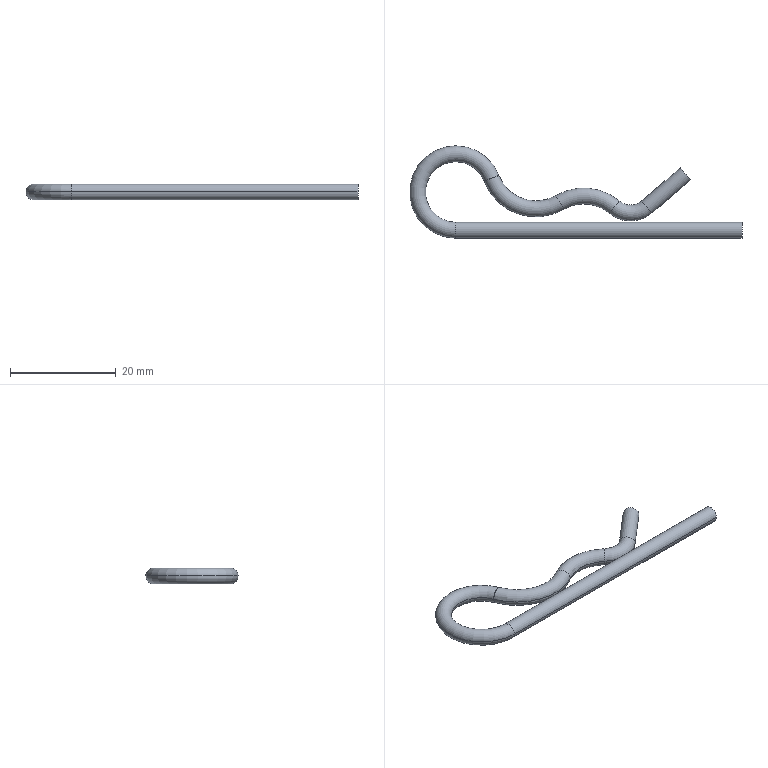Part | SolidWorks | features BaseBody 1, ICE 1, Scale 1 | 1 solid | 17 faces | box 63 x 17.5 x 3 mm | volume 910.243 mm3 | torus 8 | plane 5 | cylinder 4 | commonest cylinder face diameters 3 x4
STEP:
#1=CARTESIAN_POINT('',(9.772,3.077,0.000000307));
#2=VERTEX_POINT('',#1);
#3=CARTESIAN_POINT('',(7.84,0.7818,0.000000307));
#4=VERTEX_POINT('',#3);
#5=CARTESIAN_POINT('',(8.806,1.929,0.000000307));
#6=DIRECTION('',(0.7649,-0.6441,0.));
#7=DIRECTION('',(0.,0.,-1.));
#8=AXIS2_PLACEMENT_3D('',#5,#6,#7);
#9=CIRCLE('',#8,1.5);
#10=EDGE_CURVE('',#2,#4,#9,.T.);
#11=ORIENTED_EDGE('',*,*,#10,.T.);
#12=CARTESIAN_POINT('',(15.933,0.8171,0.000000307));
#13=VERTEX_POINT('',#12);
#14=CARTESIAN_POINT('',(11.865,5.563,0.000000307));
#15=DIRECTION('',(0.,0.,1.));
#16=DIRECTION('',(1.,0.,0.));
#17=AXIS2_PLACEMENT_3D('',#14,#15,#16);
#18=CIRCLE('',#17,6.25);
#19=EDGE_CURVE('',#4,#13,#18,.T.);
#20=ORIENTED_EDGE('',*,*,#19,.T.);
#21=CARTESIAN_POINT('',(13.98,3.095,0.000000307));
#22=VERTEX_POINT('',#21);
#23=CARTESIAN_POINT('',(14.957,1.956,0.000000307));
#24=DIRECTION('',(0.7593,0.6508,0.));
#25=DIRECTION('',(0.,0.,-1.));
#26=AXIS2_PLACEMENT_3D('',#23,#24,#25);
#27=CIRCLE('',#26,1.5);
#28=EDGE_CURVE('',#22,#13,#27,.T.);
#29=ORIENTED_EDGE('',*,*,#28,.F.);
#30=CARTESIAN_POINT('',(11.865,5.563,0.000000307));
#31=DIRECTION('',(0.,0.,1.));
#32=DIRECTION('',(1.,0.,0.));
#33=AXIS2_PLACEMENT_3D('',#30,#31,#32);
#34=CIRCLE('',#33,3.25);
#35=EDGE_CURVE('',#2,#22,#34,.T.);
#36=ORIENTED_EDGE('',*,*,#35,.F.);
#37=EDGE_LOOP('',(#11,#20,#29,#36));
#38=FACE_OUTER_BOUND('',#37,.T.);
#39=CARTESIAN_POINT('',(11.865,5.563,0.000000307));
#40=DIRECTION('',(0.,0.,1.));
#41=DIRECTION('',(-0.004363,1.,0.));
#42=AXIS2_PLACEMENT_3D('',#39,#40,#41);
#43=TOROIDAL_SURFACE('',#42,4.75,1.5);
#44=ADVANCED_FACE('',(#38),#43,.T.);
#45=CARTESIAN_POINT('',(-21.241,-0.9551,0.000000307));
#46=VERTEX_POINT('',#45);
#47=CARTESIAN_POINT('',(-21.241,-3.955,0.000000307));
#48=VERTEX_POINT('',#47);
#49=CARTESIAN_POINT('',(-21.241,-2.455,0.000000307));
#50=DIRECTION('',(-1.,0.,0.));
#51=DIRECTION('',(0.,1.,0.));
#52=AXIS2_PLACEMENT_3D('',#49,#50,#51);
#53=CIRCLE('',#52,1.5);
#54=EDGE_CURVE('',#46,#48,#53,.T.);
#55=ORIENTED_EDGE('',*,*,#54,.T.);
#56=CARTESIAN_POINT('',(-13.072,7.931,0.000000307));
#57=VERTEX_POINT('',#56);
#58=CARTESIAN_POINT('',(-21.241,4.795,0.000000307));
#59=DIRECTION('',(0.,0.,-1.));
#60=DIRECTION('',(-1.,0.,0.));
#61=AXIS2_PLACEMENT_3D('',#58,#59,#60);
#62=CIRCLE('',#61,8.75);
#63=EDGE_CURVE('',#48,#57,#62,.T.);
#64=ORIENTED_EDGE('',*,*,#63,.T.);
#65=CARTESIAN_POINT('',(-14.479,7.391,-1.5));
#66=VERTEX_POINT('',#65);
#67=CARTESIAN_POINT('',(-14.473,7.393,0.000000307));
#68=DIRECTION('',(0.3584,-0.9336,0.));
#69=DIRECTION('',(-0.9336,-0.3584,0.));
#70=AXIS2_PLACEMENT_3D('',#67,#68,#69);
#71=CIRCLE('',#70,1.5);
#72=EDGE_CURVE('',#66,#57,#71,.T.);
#73=ORIENTED_EDGE('',*,*,#72,.F.);
#74=CARTESIAN_POINT('',(-14.48,7.392,-1.5));
#75=VERTEX_POINT('',#74);
#76=CARTESIAN_POINT('',(-14.479,7.391,-1.5));
#77=DIRECTION('',(-0.3569,0.9342,-0.00000796));
#78=VECTOR('',#77,1000.);
#79=LINE('',#76,#78);
#80=EDGE_CURVE('',#66,#75,#79,.T.);
#81=ORIENTED_EDGE('',*,*,#80,.T.);
#82=CARTESIAN_POINT('',(-15.876,6.862,0.000000315));
#83=VERTEX_POINT('',#82);
#84=CARTESIAN_POINT('',(-14.48,7.392,-1.5));
#85=CARTESIAN_POINT('',(-14.662,7.323,-1.499));
#86=CARTESIAN_POINT('',(-14.845,7.254,-1.46));
#87=CARTESIAN_POINT('',(-15.183,7.125,-1.308));
#88=CARTESIAN_POINT('',(-15.338,7.067,-1.197));
#89=CARTESIAN_POINT('',(-15.597,6.968,-0.9193));
#90=CARTESIAN_POINT('',(-15.7,6.929,-0.7535));
#91=CARTESIAN_POINT('',(-15.839,6.876,-0.3914));
#92=CARTESIAN_POINT('',(-15.876,6.862,-0.1953));
#93=CARTESIAN_POINT('',(-15.876,6.862,0.000000315));
#94=B_SPLINE_CURVE_WITH_KNOTS('',3,(#84,#85,#86,#87,#88,#89,#90,#91,#92,#93),.UNSPECIFIED.,.F.,.F.,(4,2,2,2,4),(0.,0.125,0.25,0.375,0.5),.UNSPECIFIED.);
#95=EDGE_CURVE('',#75,#83,#94,.T.);
#96=ORIENTED_EDGE('',*,*,#95,.T.);
#97=CARTESIAN_POINT('',(-21.241,4.795,0.000000307));
#98=DIRECTION('',(0.,0.,-1.));
#99=DIRECTION('',(-1.,0.,0.));
#100=AXIS2_PLACEMENT_3D('',#97,#98,#99);
#101=CIRCLE('',#100,5.75);
#102=EDGE_CURVE('',#46,#83,#101,.T.);
#103=ORIENTED_EDGE('',*,*,#102,.F.);
#104=EDGE_LOOP('',(#55,#64,#73,#81,#96,#103));
#105=FACE_OUTER_BOUND('',#104,.T.);
#106=CARTESIAN_POINT('',(-21.241,4.795,0.000000307));
#107=DIRECTION('',(0.,0.,-1.));
#108=DIRECTION('',(0.8241,-0.5664,0.));
#109=AXIS2_PLACEMENT_3D('',#106,#107,#108);
#110=TOROIDAL_SURFACE('',#109,7.25,1.5);
#111=ADVANCED_FACE('',(#105),#110,.T.);
#112=CARTESIAN_POINT('',(-0.7752,1.52,0.000000307));
#113=VERTEX_POINT('',#112);
#114=CARTESIAN_POINT('',(-2.289,4.111,0.000000307));
#115=VERTEX_POINT('',#114);
#116=CARTESIAN_POINT('',(-1.532,2.815,0.000000307));
#117=DIRECTION('',(0.8634,0.5045,0.));
#118=DIRECTION('',(0.,0.,-1.));
#119=AXIS2_PLACEMENT_3D('',#116,#117,#118);
#120=CIRCLE('',#119,1.5);
#121=EDGE_CURVE('',#113,#115,#120,.T.);
#122=ORIENTED_EDGE('',*,*,#121,.F.);
#123=CARTESIAN_POINT('',(-15.888,6.857,0.000000307));
#124=VERTEX_POINT('',#123);
#125=CARTESIAN_POINT('',(-6.073,10.586,0.000000307));
#126=DIRECTION('',(0.,0.,-1.));
#127=DIRECTION('',(-1.,0.,0.));
#128=AXIS2_PLACEMENT_3D('',#125,#126,#127);
#129=CIRCLE('',#128,10.5);
#130=EDGE_CURVE('',#113,#124,#129,.T.);
#131=ORIENTED_EDGE('',*,*,#130,.T.);
#132=CARTESIAN_POINT('',(-14.486,7.39,0.000000307));
#133=DIRECTION('',(-0.3551,0.9348,0.));
#134=DIRECTION('',(0.,0.,1.));
#135=AXIS2_PLACEMENT_3D('',#132,#133,#134);
#136=CIRCLE('',#135,1.5);
#137=EDGE_CURVE('',#75,#124,#136,.T.);
#138=ORIENTED_EDGE('',*,*,#137,.F.);
#139=ORIENTED_EDGE('',*,*,#80,.F.);
#140=CARTESIAN_POINT('',(-13.954,7.592,-1.388));
#141=VERTEX_POINT('',#140);
#142=CARTESIAN_POINT('',(-13.954,7.592,-1.388));
#143=CARTESIAN_POINT('',(-14.119,7.529,-1.46));
#144=CARTESIAN_POINT('',(-14.3,7.459,-1.499));
#145=CARTESIAN_POINT('',(-14.479,7.391,-1.5));
#146=B_SPLINE_CURVE_WITH_KNOTS('',3,(#142,#143,#144,#145),.UNSPECIFIED.,.F.,.F.,(4,4),(0.,1.),.UNSPECIFIED.);
#147=EDGE_CURVE('',#141,#66,#146,.T.);
#148=ORIENTED_EDGE('',*,*,#147,.F.);
#149=CARTESIAN_POINT('',(-13.084,7.923,0.000000307));
#150=VERTEX_POINT('',#149);
#151=CARTESIAN_POINT('',(-14.486,7.39,0.000000307));
#152=DIRECTION('',(-0.3551,0.9348,0.));
#153=DIRECTION('',(0.,0.,1.));
#154=AXIS2_PLACEMENT_3D('',#151,#152,#153);
#155=CIRCLE('',#154,1.5);
#156=EDGE_CURVE('',#150,#141,#155,.T.);
#157=ORIENTED_EDGE('',*,*,#156,.F.);
#158=CARTESIAN_POINT('',(-6.073,10.586,0.000000307));
#159=DIRECTION('',(0.,0.,-1.));
#160=DIRECTION('',(-1.,0.,0.));
#161=AXIS2_PLACEMENT_3D('',#158,#159,#160);
#162=CIRCLE('',#161,7.5);
#163=EDGE_CURVE('',#115,#150,#162,.T.);
#164=ORIENTED_EDGE('',*,*,#163,.F.);
#165=EDGE_LOOP('',(#122,#131,#138,#139,#148,#157,#164));
#166=FACE_OUTER_BOUND('',#165,.T.);
#167=CARTESIAN_POINT('',(-6.073,10.586,0.000000307));
#168=DIRECTION('',(0.,0.,-1.));
#169=DIRECTION('',(0.333,0.9429,0.));
#170=AXIS2_PLACEMENT_3D('',#167,#168,#169);
#171=TOROIDAL_SURFACE('',#170,9.,1.5);
#172=ADVANCED_FACE('',(#166),#171,.T.);
#173=ORIENTED_EDGE('',*,*,#121,.T.);
#174=CARTESIAN_POINT('',(3.009,-4.955,0.000000307));
#175=DIRECTION('',(0.,0.,-1.));
#176=DIRECTION('',(-1.,0.,0.));
#177=AXIS2_PLACEMENT_3D('',#174,#175,#176);
#178=CIRCLE('',#177,10.5);
#179=EDGE_CURVE('',#115,#2,#178,.T.);
#180=ORIENTED_EDGE('',*,*,#179,.T.);
#181=CARTESIAN_POINT('',(8.806,1.929,0.000000307));
#182=DIRECTION('',(0.7649,-0.6441,0.));
#183=DIRECTION('',(0.,0.,-1.));
#184=AXIS2_PLACEMENT_3D('',#181,#182,#183);
#185=CIRCLE('',#184,1.5);
#186=EDGE_CURVE('',#4,#2,#185,.T.);
#187=ORIENTED_EDGE('',*,*,#186,.F.);
#188=CARTESIAN_POINT('',(3.009,-4.955,0.000000307));
#189=DIRECTION('',(0.,0.,-1.));
#190=DIRECTION('',(-1.,0.,0.));
#191=AXIS2_PLACEMENT_3D('',#188,#189,#190);
#192=CIRCLE('',#191,7.5);
#193=EDGE_CURVE('',#113,#4,#192,.T.);
#194=ORIENTED_EDGE('',*,*,#193,.F.);
#195=EDGE_LOOP('',(#173,#180,#187,#194));
#196=FACE_OUTER_BOUND('',#195,.T.);
#197=CARTESIAN_POINT('',(3.009,-4.955,0.000000307));
#198=DIRECTION('',(0.,0.,-1.));
#199=DIRECTION('',(-0.08542,-0.9963,0.));
#200=AXIS2_PLACEMENT_3D('',#197,#198,#199);
#201=TOROIDAL_SURFACE('',#200,9.,1.5);
#202=ADVANCED_FACE('',(#196),#201,.T.);
#203=CARTESIAN_POINT('',(21.299,9.368,0.000000307));
#204=VERTEX_POINT('',#203);
#205=CARTESIAN_POINT('',(23.252,7.09,0.000000307));
#206=VERTEX_POINT('',#205);
#207=CARTESIAN_POINT('',(22.276,8.229,0.000000307));
#208=DIRECTION('',(0.7593,0.6508,0.));
#209=DIRECTION('',(-0.6508,0.7593,0.));
#210=AXIS2_PLACEMENT_3D('',#207,#208,#209);
#211=CIRCLE('',#210,1.5);
#212=EDGE_CURVE('',#204,#206,#211,.T.);
#213=ORIENTED_EDGE('',*,*,#212,.F.);
#214=CARTESIAN_POINT('',(21.299,9.368,0.000000307));
#215=DIRECTION('',(-0.7593,-0.6508,0.));
#216=VECTOR('',#215,1000.);
#217=LINE('',#214,#216);
#218=EDGE_CURVE('',#204,#22,#217,.T.);
#219=ORIENTED_EDGE('',*,*,#218,.T.);
#220=ORIENTED_EDGE('',*,*,#28,.T.);
#221=CARTESIAN_POINT('',(23.252,7.09,0.000000307));
#222=DIRECTION('',(-0.7593,-0.6508,0.));
#223=VECTOR('',#222,1000.);
#224=LINE('',#221,#223);
#225=EDGE_CURVE('',#206,#13,#224,.T.);
#226=ORIENTED_EDGE('',*,*,#225,.F.);
#227=EDGE_LOOP('',(#213,#219,#220,#226));
#228=FACE_OUTER_BOUND('',#227,.T.);
#229=CARTESIAN_POINT('',(22.276,8.229,0.000000307));
#230=DIRECTION('',(-0.7593,-0.6508,0.));
#231=DIRECTION('',(0.6508,-0.7593,0.));
#232=AXIS2_PLACEMENT_3D('',#229,#230,#231);
#233=CYLINDRICAL_SURFACE('',#232,1.5);
#234=ADVANCED_FACE('',(#228),#233,.T.);
#235=CARTESIAN_POINT('',(33.009,-0.9551,0.000000307));
#236=VERTEX_POINT('',#235);
#237=CARTESIAN_POINT('',(33.009,-3.955,0.000000307));
#238=VERTEX_POINT('',#237);
#239=CARTESIAN_POINT('',(33.009,-2.455,0.000000307));
#240=DIRECTION('',(-1.,0.,0.));
#241=DIRECTION('',(0.,0.,1.));
#242=AXIS2_PLACEMENT_3D('',#239,#240,#241);
#243=CIRCLE('',#242,1.5);
#244=EDGE_CURVE('',#236,#238,#243,.T.);
#245=ORIENTED_EDGE('',*,*,#244,.T.);
#246=CARTESIAN_POINT('',(-21.241,-3.955,0.000000307));
#247=DIRECTION('',(-1.,0.,0.));
#248=VECTOR('',#247,1000.);
#249=LINE('',#246,#248);
#250=EDGE_CURVE('',#238,#48,#249,.T.);
#251=ORIENTED_EDGE('',*,*,#250,.T.);
#252=ORIENTED_EDGE('',*,*,#54,.F.);
#253=CARTESIAN_POINT('',(-21.241,-0.9551,0.000000307));
#254=DIRECTION('',(-1.,0.,0.));
#255=VECTOR('',#254,1000.);
#256=LINE('',#253,#255);
#257=EDGE_CURVE('',#236,#46,#256,.T.);
#258=ORIENTED_EDGE('',*,*,#257,.F.);
#259=EDGE_LOOP('',(#245,#251,#252,#258));
#260=FACE_OUTER_BOUND('',#259,.T.);
#261=CARTESIAN_POINT('',(-21.241,-2.455,0.000000307));
#262=DIRECTION('',(-1.,0.,0.));
#263=DIRECTION('',(0.,1.,0.));
#264=AXIS2_PLACEMENT_3D('',#261,#262,#263);
#265=CYLINDRICAL_SURFACE('',#264,1.5);
#266=ADVANCED_FACE('',(#260),#265,.T.);
#267=CARTESIAN_POINT('',(-14.907,7.23,1.427));
#268=VERTEX_POINT('',#267);
#269=CARTESIAN_POINT('',(-14.48,7.392,1.5));
#270=VERTEX_POINT('',#269);
#271=CARTESIAN_POINT('',(-14.907,7.23,1.427));
#272=CARTESIAN_POINT('',(-14.769,7.283,1.474));
#273=CARTESIAN_POINT('',(-14.625,7.337,1.499));
#274=CARTESIAN_POINT('',(-14.48,7.392,1.5));
#275=B_SPLINE_CURVE_WITH_KNOTS('',3,(#271,#272,#273,#274),.UNSPECIFIED.,.F.,.F.,(4,4),(0.,0.3096),.UNSPECIFIED.);
#276=EDGE_CURVE('',#268,#270,#275,.T.);
#277=ORIENTED_EDGE('',*,*,#276,.F.);
#278=CARTESIAN_POINT('',(-15.876,6.862,0.000000315));
#279=CARTESIAN_POINT('',(-15.876,6.862,0.3133));
#280=CARTESIAN_POINT('',(-15.781,6.898,0.6276));
#281=CARTESIAN_POINT('',(-15.435,7.03,1.136));
#282=CARTESIAN_POINT('',(-15.187,7.124,1.329));
#283=CARTESIAN_POINT('',(-14.907,7.23,1.427));
#284=B_SPLINE_CURVE_WITH_KNOTS('',3,(#278,#279,#280,#281,#282,#283),.UNSPECIFIED.,.F.,.F.,(4,2,4),(0.5,0.7005,0.9011),.UNSPECIFIED.);
#285=EDGE_CURVE('',#83,#268,#284,.T.);
#286=ORIENTED_EDGE('',*,*,#285,.F.);
#287=ORIENTED_EDGE('',*,*,#95,.F.);
#288=ORIENTED_EDGE('',*,*,#137,.T.);
#289=CARTESIAN_POINT('',(-14.486,7.39,0.000000307));
#290=DIRECTION('',(-0.3551,0.9348,0.));
#291=DIRECTION('',(0.,0.,1.));
#292=AXIS2_PLACEMENT_3D('',#289,#290,#291);
#293=CIRCLE('',#292,1.5);
#294=EDGE_CURVE('',#124,#270,#293,.T.);
#295=ORIENTED_EDGE('',*,*,#294,.T.);
#296=EDGE_LOOP('',(#277,#286,#287,#288,#295));
#297=FACE_OUTER_BOUND('',#296,.T.);
#298=CARTESIAN_POINT('',(-14.486,7.39,0.000000307));
#299=DIRECTION('',(-0.3551,0.9348,0.));
#300=DIRECTION('',(-0.9348,-0.3551,0.));
#301=AXIS2_PLACEMENT_3D('',#298,#299,#300);
#302=PLANE('',#301);
#303=ADVANCED_FACE('',(#297),#302,.T.);
#304=ORIENTED_EDGE('',*,*,#179,.F.);
#305=CARTESIAN_POINT('',(-1.532,2.815,0.000000307));
#306=DIRECTION('',(0.8634,0.5045,0.));
#307=DIRECTION('',(0.,0.,-1.));
#308=AXIS2_PLACEMENT_3D('',#305,#306,#307);
#309=CIRCLE('',#308,1.5);
#310=EDGE_CURVE('',#115,#113,#309,.T.);
#311=ORIENTED_EDGE('',*,*,#310,.T.);
#312=ORIENTED_EDGE('',*,*,#193,.T.);
#313=ORIENTED_EDGE('',*,*,#10,.F.);
#314=EDGE_LOOP('',(#304,#311,#312,#313));
#315=FACE_OUTER_BOUND('',#314,.T.);
#316=CARTESIAN_POINT('',(3.009,-4.955,0.000000307));
#317=DIRECTION('',(0.,0.,-1.));
#318=DIRECTION('',(-0.08542,-0.9963,0.));
#319=AXIS2_PLACEMENT_3D('',#316,#317,#318);
#320=TOROIDAL_SURFACE('',#319,9.,1.5);
#321=ADVANCED_FACE('',(#315),#320,.T.);
#322=ORIENTED_EDGE('',*,*,#130,.F.);
#323=ORIENTED_EDGE('',*,*,#310,.F.);
#324=ORIENTED_EDGE('',*,*,#163,.T.);
#325=CARTESIAN_POINT('',(-13.954,7.592,1.388));
#326=VERTEX_POINT('',#325);
#327=CARTESIAN_POINT('',(-14.486,7.39,0.000000307));
#328=DIRECTION('',(-0.3551,0.9348,0.));
#329=DIRECTION('',(0.,0.,1.));
#330=AXIS2_PLACEMENT_3D('',#327,#328,#329);
#331=CIRCLE('',#330,1.5);
#332=EDGE_CURVE('',#326,#150,#331,.T.);
#333=ORIENTED_EDGE('',*,*,#332,.F.);
#334=CARTESIAN_POINT('',(-14.053,7.554,1.427));
#335=VERTEX_POINT('',#334);
#336=CARTESIAN_POINT('',(-14.053,7.554,1.427));
#337=CARTESIAN_POINT('',(-14.019,7.567,1.415));
#338=CARTESIAN_POINT('',(-13.986,7.58,1.402));
#339=CARTESIAN_POINT('',(-13.954,7.592,1.388));
#340=B_SPLINE_CURVE_WITH_KNOTS('',3,(#336,#337,#338,#339),.UNSPECIFIED.,.F.,.F.,(4,4),(0.8052,1.),.UNSPECIFIED.);
#341=EDGE_CURVE('',#335,#326,#340,.T.);
#342=ORIENTED_EDGE('',*,*,#341,.F.);
#343=CARTESIAN_POINT('',(-14.479,7.391,1.5));
#344=VERTEX_POINT('',#343);
#345=CARTESIAN_POINT('',(-14.479,7.391,1.5));
#346=CARTESIAN_POINT('',(-14.335,7.446,1.499));
#347=CARTESIAN_POINT('',(-14.191,7.501,1.475));
#348=CARTESIAN_POINT('',(-14.053,7.554,1.427));
#349=B_SPLINE_CURVE_WITH_KNOTS('',3,(#345,#346,#347,#348),.UNSPECIFIED.,.F.,.F.,(4,4),(0.,0.8052),.UNSPECIFIED.);
#350=EDGE_CURVE('',#344,#335,#349,.T.);
#351=ORIENTED_EDGE('',*,*,#350,.F.);
#352=CARTESIAN_POINT('',(-14.48,7.392,1.5));
#353=DIRECTION('',(0.3569,-0.9342,-0.00000796));
#354=VECTOR('',#353,1000.);
#355=LINE('',#352,#354);
#356=EDGE_CURVE('',#270,#344,#355,.T.);
#357=ORIENTED_EDGE('',*,*,#356,.F.);
#358=ORIENTED_EDGE('',*,*,#294,.F.);
#359=EDGE_LOOP('',(#322,#323,#324,#333,#342,#351,#357,#358));
#360=FACE_OUTER_BOUND('',#359,.T.);
#361=CARTESIAN_POINT('',(-6.073,10.586,0.000000307));
#362=DIRECTION('',(0.,0.,-1.));
#363=DIRECTION('',(0.333,0.9429,0.));
#364=AXIS2_PLACEMENT_3D('',#361,#362,#363);
#365=TOROIDAL_SURFACE('',#364,9.,1.5);
#366=ADVANCED_FACE('',(#360),#365,.T.);
#367=CARTESIAN_POINT('',(-13.954,7.592,1.388));
#368=CARTESIAN_POINT('',(-13.954,7.592,0.4626));
#369=CARTESIAN_POINT('',(-13.954,7.592,-0.4626));
#370=CARTESIAN_POINT('',(-13.954,7.592,-1.388));
#371=B_SPLINE_CURVE_WITH_KNOTS('',3,(#367,#368,#369,#370),.UNSPECIFIED.,.F.,.F.,(4,4),(-0.5551,0.5551),.UNSPECIFIED.);
#372=EDGE_CURVE('',#326,#141,#371,.T.);
#373=ORIENTED_EDGE('',*,*,#372,.T.);
#374=ORIENTED_EDGE('',*,*,#147,.T.);
#375=ORIENTED_EDGE('',*,*,#72,.T.);
#376=CARTESIAN_POINT('',(-14.473,7.393,0.000000307));
#377=DIRECTION('',(0.3584,-0.9336,0.));
#378=DIRECTION('',(-0.9336,-0.3584,0.));
#379=AXIS2_PLACEMENT_3D('',#376,#377,#378);
#380=CIRCLE('',#379,1.5);
#381=EDGE_CURVE('',#57,#344,#380,.T.);
#382=ORIENTED_EDGE('',*,*,#381,.T.);
#383=ORIENTED_EDGE('',*,*,#350,.T.);
#384=ORIENTED_EDGE('',*,*,#341,.T.);
#385=EDGE_LOOP('',(#373,#374,#375,#382,#383,#384));
#386=FACE_OUTER_BOUND('',#385,.T.);
#387=CARTESIAN_POINT('',(-14.473,7.393,0.000000307));
#388=DIRECTION('',(0.3584,-0.9336,0.));
#389=DIRECTION('',(0.,0.,1.));
#390=AXIS2_PLACEMENT_3D('',#387,#388,#389);
#391=PLANE('',#390);
#392=ADVANCED_FACE('',(#386),#391,.T.);
#393=ORIENTED_EDGE('',*,*,#244,.F.);
#394=CARTESIAN_POINT('',(33.009,-2.455,0.000000307));
#395=DIRECTION('',(-1.,0.,0.));
#396=DIRECTION('',(0.,0.,1.));
#397=AXIS2_PLACEMENT_3D('',#394,#395,#396);
#398=CIRCLE('',#397,1.5);
#399=EDGE_CURVE('',#238,#236,#398,.T.);
#400=ORIENTED_EDGE('',*,*,#399,.F.);
#401=EDGE_LOOP('',(#393,#400));
#402=FACE_OUTER_BOUND('',#401,.T.);
#403=CARTESIAN_POINT('',(33.009,-2.455,0.000000307));
#404=DIRECTION('',(-1.,0.,0.));
#405=DIRECTION('',(0.,0.,1.));
#406=AXIS2_PLACEMENT_3D('',#403,#404,#405);
#407=PLANE('',#406);
#408=ADVANCED_FACE('',(#402),#407,.F.);
#409=ORIENTED_EDGE('',*,*,#250,.F.);
#410=ORIENTED_EDGE('',*,*,#399,.T.);
#411=ORIENTED_EDGE('',*,*,#257,.T.);
#412=CARTESIAN_POINT('',(-21.241,-2.455,0.000000307));
#413=DIRECTION('',(-1.,0.,0.));
#414=DIRECTION('',(0.,1.,0.));
#415=AXIS2_PLACEMENT_3D('',#412,#413,#414);
#416=CIRCLE('',#415,1.5);
#417=EDGE_CURVE('',#48,#46,#416,.T.);
#418=ORIENTED_EDGE('',*,*,#417,.F.);
#419=EDGE_LOOP('',(#409,#410,#411,#418));
#420=FACE_OUTER_BOUND('',#419,.T.);
#421=CARTESIAN_POINT('',(-21.241,-2.455,0.000000307));
#422=DIRECTION('',(-1.,0.,0.));
#423=DIRECTION('',(0.,1.,0.));
#424=AXIS2_PLACEMENT_3D('',#421,#422,#423);
#425=CYLINDRICAL_SURFACE('',#424,1.5);
#426=ADVANCED_FACE('',(#420),#425,.T.);
#427=ORIENTED_EDGE('',*,*,#63,.F.);
#428=ORIENTED_EDGE('',*,*,#417,.T.);
#429=ORIENTED_EDGE('',*,*,#102,.T.);
#430=ORIENTED_EDGE('',*,*,#285,.T.);
#431=ORIENTED_EDGE('',*,*,#276,.T.);
#432=ORIENTED_EDGE('',*,*,#356,.T.);
#433=ORIENTED_EDGE('',*,*,#381,.F.);
#434=EDGE_LOOP('',(#427,#428,#429,#430,#431,#432,#433));
#435=FACE_OUTER_BOUND('',#434,.T.);
#436=CARTESIAN_POINT('',(-21.241,4.795,0.000000307));
#437=DIRECTION('',(0.,0.,-1.));
#438=DIRECTION('',(0.8241,-0.5664,0.));
#439=AXIS2_PLACEMENT_3D('',#436,#437,#438);
#440=TOROIDAL_SURFACE('',#439,7.25,1.5);
#441=ADVANCED_FACE('',(#435),#440,.T.);
#442=ORIENTED_EDGE('',*,*,#372,.F.);
#443=ORIENTED_EDGE('',*,*,#332,.T.);
#444=ORIENTED_EDGE('',*,*,#156,.T.);
#445=EDGE_LOOP('',(#442,#443,#444));
#446=FACE_OUTER_BOUND('',#445,.T.);
#447=CARTESIAN_POINT('',(-14.486,7.39,0.000000307));
#448=DIRECTION('',(-0.3551,0.9348,0.));
#449=DIRECTION('',(-0.9348,-0.3551,0.));
#450=AXIS2_PLACEMENT_3D('',#447,#448,#449);
#451=PLANE('',#450);
#452=ADVANCED_FACE('',(#446),#451,.T.);
#453=ORIENTED_EDGE('',*,*,#19,.F.);
#454=ORIENTED_EDGE('',*,*,#186,.T.);
#455=ORIENTED_EDGE('',*,*,#35,.T.);
#456=CARTESIAN_POINT('',(14.957,1.956,0.000000307));
#457=DIRECTION('',(0.7593,0.6508,0.));
#458=DIRECTION('',(0.,0.,-1.));
#459=AXIS2_PLACEMENT_3D('',#456,#457,#458);
#460=CIRCLE('',#459,1.5);
#461=EDGE_CURVE('',#13,#22,#460,.T.);
#462=ORIENTED_EDGE('',*,*,#461,.F.);
#463=EDGE_LOOP('',(#453,#454,#455,#462));
#464=FACE_OUTER_BOUND('',#463,.T.);
#465=CARTESIAN_POINT('',(11.865,5.563,0.000000307));
#466=DIRECTION('',(0.,0.,1.));
#467=DIRECTION('',(-0.004363,1.,0.));
#468=AXIS2_PLACEMENT_3D('',#465,#466,#467);
#469=TOROIDAL_SURFACE('',#468,4.75,1.5);
#470=ADVANCED_FACE('',(#464),#469,.T.);
#471=ORIENTED_EDGE('',*,*,#218,.F.);
#472=CARTESIAN_POINT('',(22.276,8.229,0.000000307));
#473=DIRECTION('',(0.7593,0.6508,0.));
#474=DIRECTION('',(-0.6508,0.7593,0.));
#475=AXIS2_PLACEMENT_3D('',#472,#473,#474);
#476=CIRCLE('',#475,1.5);
#477=EDGE_CURVE('',#206,#204,#476,.T.);
#478=ORIENTED_EDGE('',*,*,#477,.F.);
#479=ORIENTED_EDGE('',*,*,#225,.T.);
#480=ORIENTED_EDGE('',*,*,#461,.T.);
#481=EDGE_LOOP('',(#471,#478,#479,#480));
#482=FACE_OUTER_BOUND('',#481,.T.);
#483=CARTESIAN_POINT('',(22.276,8.229,0.000000307));
#484=DIRECTION('',(-0.7593,-0.6508,0.));
#485=DIRECTION('',(0.6508,-0.7593,0.));
#486=AXIS2_PLACEMENT_3D('',#483,#484,#485);
#487=CYLINDRICAL_SURFACE('',#486,1.5);
#488=ADVANCED_FACE('',(#482),#487,.T.);
#489=ORIENTED_EDGE('',*,*,#477,.T.);
#490=ORIENTED_EDGE('',*,*,#212,.T.);
#491=EDGE_LOOP('',(#489,#490));
#492=FACE_OUTER_BOUND('',#491,.T.);
#493=CARTESIAN_POINT('',(22.276,8.229,0.000000307));
#494=DIRECTION('',(0.7593,0.6508,0.));
#495=DIRECTION('',(-0.6508,0.7593,0.));
#496=AXIS2_PLACEMENT_3D('',#493,#494,#495);
#497=PLANE('',#496);
#498=ADVANCED_FACE('',(#492),#497,.T.);
#499=CLOSED_SHELL('',(#44,#111,#172,#202,#234,#266,#303,#321,#366,#392,#408,#426,#441,#452,#470,#488,#498));
#500=MANIFOLD_SOLID_BREP('',#499);
#501=CARTESIAN_POINT('',(0.,0.,0.));
#502=DIRECTION('',(0.,0.,1.));
#503=DIRECTION('',(1.,0.,0.));
#504=AXIS2_PLACEMENT_3D('',#501,#502,#503);
#505=(LENGTH_UNIT()NAMED_UNIT(*)SI_UNIT(.MILLI.,.METRE.));
#506=UNCERTAINTY_MEASURE_WITH_UNIT(LENGTH_MEASURE(0.00001),#505,'','');
#507=(NAMED_UNIT(*)PLANE_ANGLE_UNIT()SI_UNIT($,.RADIAN.));
#508=(NAMED_UNIT(*)SI_UNIT($,.STERADIAN.)SOLID_ANGLE_UNIT());
#509=(GEOMETRIC_REPRESENTATION_CONTEXT(3)GLOBAL_UNCERTAINTY_ASSIGNED_CONTEXT((#506))GLOBAL_UNIT_ASSIGNED_CONTEXT((#505,#507,#508))REPRESENTATION_CONTEXT('',''));
#510=ADVANCED_BREP_SHAPE_REPRESENTATION('',(#500,#504),#509);